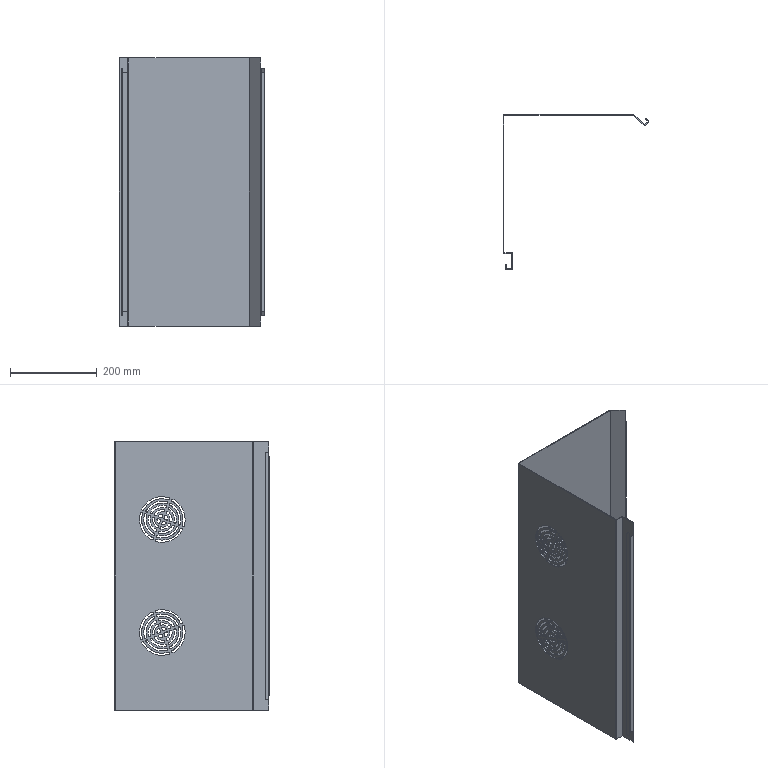Part | SolidWorks | features SMBaseFlange 3, EdgeFlange 2, Fillet 1, FlatPattern 1, MacroFeature 1, MirrorPattern 1, SheetMetal 1 | 1 solid | 446 faces | box 334.929 x 356.5 x 617 mm | volume 679567 mm3 | cylinder 212 | plane 146 | spline 88 | commonest cylinder face diameters 4 x192 0.2 x8 3.2 x8 10 x4